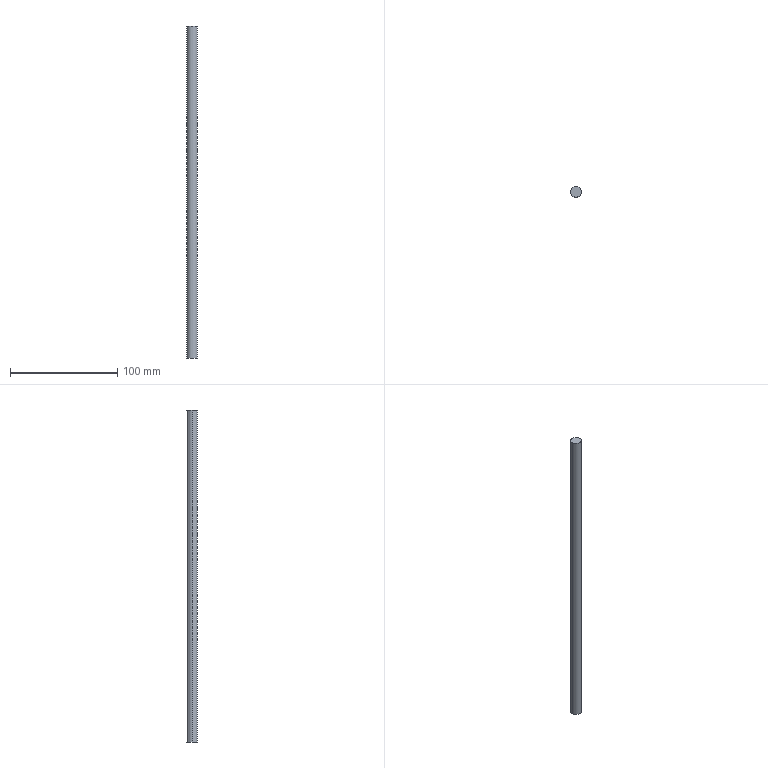Part | STEP file | 1 solid | 4 faces | box 10 x 10 x 310 mm | volume 24347 mm3 | cylinder 2 | plane 2 | commonest cylinder face diameters 10 x2
STEP:
#1=CARTESIAN_POINT('',(0.,0.,0.));
#2=DIRECTION('',(0.,0.,1.));
#3=DIRECTION('',(1.,0.,0.));
#4=AXIS2_PLACEMENT_3D('',#1,#2,#3);
#5=CARTESIAN_POINT('',(5.,0.,310.));
#6=VERTEX_POINT('',#5);
#7=CARTESIAN_POINT('',(-5.,0.,310.));
#8=VERTEX_POINT('',#7);
#9=CARTESIAN_POINT('',(0.,0.,310.));
#10=DIRECTION('',(0.,0.,1.));
#11=DIRECTION('',(1.,0.,0.));
#12=AXIS2_PLACEMENT_3D('',#9,#10,#11);
#13=CIRCLE('',#12,5.);
#14=CARTESIAN_POINT('',(0.,0.,310.));
#15=DIRECTION('',(0.,0.,-1.));
#16=DIRECTION('',(-1.,0.,0.));
#17=AXIS2_PLACEMENT_3D('',#14,#15,#16);
#18=CYLINDRICAL_SURFACE('',#17,5.);
#19=CARTESIAN_POINT('',(3.142,0.));
#20=DIRECTION('',(-1.,0.));
#21=VECTOR('',#20,1.);
#22=LINE('',#19,#21);
#23=(GEOMETRIC_REPRESENTATION_CONTEXT(2)PARAMETRIC_REPRESENTATION_CONTEXT()REPRESENTATION_CONTEXT('',''));
#24=DEFINITIONAL_REPRESENTATION('',(#22),#23);
#25=PCURVE('',#18,#24);
#26=CARTESIAN_POINT('',(0.,0.,310.));
#27=DIRECTION('',(0.,0.,1.));
#28=DIRECTION('',(1.,0.,0.));
#29=AXIS2_PLACEMENT_3D('',#26,#27,#28);
#30=PLANE('',#29);
#31=CARTESIAN_POINT('',(0.,0.));
#32=DIRECTION('',(1.,0.));
#33=AXIS2_PLACEMENT_2D('',#31,#32);
#34=CIRCLE('',#33,5.);
#35=(GEOMETRIC_REPRESENTATION_CONTEXT(2)PARAMETRIC_REPRESENTATION_CONTEXT()REPRESENTATION_CONTEXT('',''));
#36=DEFINITIONAL_REPRESENTATION('',(#34),#35);
#37=PCURVE('',#30,#36);
#38=SURFACE_CURVE('',#13,(#25,#37),.PCURVE_S1.);
#39=EDGE_CURVE('',#6,#8,#38,.T.);
#40=ORIENTED_EDGE('',*,*,#39,.F.);
#41=CARTESIAN_POINT('',(5.,0.,0.));
#42=VERTEX_POINT('',#41);
#43=CARTESIAN_POINT('',(5.,0.,310.));
#44=DIRECTION('',(0.,0.,-1.));
#45=VECTOR('',#44,1.);
#46=LINE('',#43,#45);
#47=CARTESIAN_POINT('',(3.142,0.));
#48=DIRECTION('',(0.,1.));
#49=VECTOR('',#48,1.);
#50=LINE('',#47,#49);
#51=(GEOMETRIC_REPRESENTATION_CONTEXT(2)PARAMETRIC_REPRESENTATION_CONTEXT()REPRESENTATION_CONTEXT('',''));
#52=DEFINITIONAL_REPRESENTATION('',(#50),#51);
#53=PCURVE('',#18,#52);
#54=CARTESIAN_POINT('',(0.,0.,310.));
#55=DIRECTION('',(0.,0.,-1.));
#56=DIRECTION('',(-1.,0.,0.));
#57=AXIS2_PLACEMENT_3D('',#54,#55,#56);
#58=CYLINDRICAL_SURFACE('',#57,5.);
#59=CARTESIAN_POINT('',(3.142,0.));
#60=DIRECTION('',(0.,1.));
#61=VECTOR('',#60,1.);
#62=LINE('',#59,#61);
#63=(GEOMETRIC_REPRESENTATION_CONTEXT(2)PARAMETRIC_REPRESENTATION_CONTEXT()REPRESENTATION_CONTEXT('',''));
#64=DEFINITIONAL_REPRESENTATION('',(#62),#63);
#65=PCURVE('',#58,#64);
#66=SURFACE_CURVE('',#46,(#53,#65),.PCURVE_S1.);
#67=EDGE_CURVE('',#6,#42,#66,.T.);
#68=ORIENTED_EDGE('',*,*,#67,.T.);
#69=CARTESIAN_POINT('',(-5.,0.,0.));
#70=VERTEX_POINT('',#69);
#71=CARTESIAN_POINT('',(0.,0.,0.));
#72=DIRECTION('',(0.,0.,1.));
#73=DIRECTION('',(1.,0.,0.));
#74=AXIS2_PLACEMENT_3D('',#71,#72,#73);
#75=CIRCLE('',#74,5.);
#76=CARTESIAN_POINT('',(3.142,310.));
#77=DIRECTION('',(-1.,0.));
#78=VECTOR('',#77,1.);
#79=LINE('',#76,#78);
#80=(GEOMETRIC_REPRESENTATION_CONTEXT(2)PARAMETRIC_REPRESENTATION_CONTEXT()REPRESENTATION_CONTEXT('',''));
#81=DEFINITIONAL_REPRESENTATION('',(#79),#80);
#82=PCURVE('',#18,#81);
#83=CARTESIAN_POINT('',(0.,0.,0.));
#84=DIRECTION('',(0.,0.,1.));
#85=DIRECTION('',(1.,0.,0.));
#86=AXIS2_PLACEMENT_3D('',#83,#84,#85);
#87=PLANE('',#86);
#88=CARTESIAN_POINT('',(0.,0.));
#89=DIRECTION('',(1.,0.));
#90=AXIS2_PLACEMENT_2D('',#88,#89);
#91=CIRCLE('',#90,5.);
#92=(GEOMETRIC_REPRESENTATION_CONTEXT(2)PARAMETRIC_REPRESENTATION_CONTEXT()REPRESENTATION_CONTEXT('',''));
#93=DEFINITIONAL_REPRESENTATION('',(#91),#92);
#94=PCURVE('',#87,#93);
#95=SURFACE_CURVE('',#75,(#82,#94),.PCURVE_S1.);
#96=EDGE_CURVE('',#42,#70,#95,.T.);
#97=ORIENTED_EDGE('',*,*,#96,.T.);
#98=CARTESIAN_POINT('',(-5.,0.,310.));
#99=DIRECTION('',(0.,0.,-1.));
#100=VECTOR('',#99,1.);
#101=LINE('',#98,#100);
#102=CARTESIAN_POINT('',(0.,0.));
#103=DIRECTION('',(0.,1.));
#104=VECTOR('',#103,1.);
#105=LINE('',#102,#104);
#106=(GEOMETRIC_REPRESENTATION_CONTEXT(2)PARAMETRIC_REPRESENTATION_CONTEXT()REPRESENTATION_CONTEXT('',''));
#107=DEFINITIONAL_REPRESENTATION('',(#105),#106);
#108=PCURVE('',#18,#107);
#109=CARTESIAN_POINT('',(6.283,0.));
#110=DIRECTION('',(0.,1.));
#111=VECTOR('',#110,1.);
#112=LINE('',#109,#111);
#113=(GEOMETRIC_REPRESENTATION_CONTEXT(2)PARAMETRIC_REPRESENTATION_CONTEXT()REPRESENTATION_CONTEXT('',''));
#114=DEFINITIONAL_REPRESENTATION('',(#112),#113);
#115=PCURVE('',#58,#114);
#116=SURFACE_CURVE('',#101,(#108,#115),.PCURVE_S1.);
#117=EDGE_CURVE('',#8,#70,#116,.T.);
#118=ORIENTED_EDGE('',*,*,#117,.F.);
#119=EDGE_LOOP('',(#40,#68,#97,#118));
#120=FACE_BOUND('',#119,.T.);
#121=ADVANCED_FACE('',(#120),#18,.T.);
#122=ORIENTED_EDGE('',*,*,#67,.F.);
#123=CARTESIAN_POINT('',(0.,0.,310.));
#124=DIRECTION('',(0.,0.,1.));
#125=DIRECTION('',(1.,0.,0.));
#126=AXIS2_PLACEMENT_3D('',#123,#124,#125);
#127=CIRCLE('',#126,5.);
#128=CARTESIAN_POINT('',(9.425,0.));
#129=DIRECTION('',(-1.,0.));
#130=VECTOR('',#129,1.);
#131=LINE('',#128,#130);
#132=(GEOMETRIC_REPRESENTATION_CONTEXT(2)PARAMETRIC_REPRESENTATION_CONTEXT()REPRESENTATION_CONTEXT('',''));
#133=DEFINITIONAL_REPRESENTATION('',(#131),#132);
#134=PCURVE('',#58,#133);
#135=CARTESIAN_POINT('',(0.,0.));
#136=DIRECTION('',(1.,0.));
#137=AXIS2_PLACEMENT_2D('',#135,#136);
#138=CIRCLE('',#137,5.);
#139=(GEOMETRIC_REPRESENTATION_CONTEXT(2)PARAMETRIC_REPRESENTATION_CONTEXT()REPRESENTATION_CONTEXT('',''));
#140=DEFINITIONAL_REPRESENTATION('',(#138),#139);
#141=PCURVE('',#30,#140);
#142=SURFACE_CURVE('',#127,(#134,#141),.PCURVE_S1.);
#143=EDGE_CURVE('',#8,#6,#142,.T.);
#144=ORIENTED_EDGE('',*,*,#143,.F.);
#145=ORIENTED_EDGE('',*,*,#117,.T.);
#146=CARTESIAN_POINT('',(0.,0.,0.));
#147=DIRECTION('',(0.,0.,1.));
#148=DIRECTION('',(1.,0.,0.));
#149=AXIS2_PLACEMENT_3D('',#146,#147,#148);
#150=CIRCLE('',#149,5.);
#151=CARTESIAN_POINT('',(9.425,310.));
#152=DIRECTION('',(-1.,0.));
#153=VECTOR('',#152,1.);
#154=LINE('',#151,#153);
#155=(GEOMETRIC_REPRESENTATION_CONTEXT(2)PARAMETRIC_REPRESENTATION_CONTEXT()REPRESENTATION_CONTEXT('',''));
#156=DEFINITIONAL_REPRESENTATION('',(#154),#155);
#157=PCURVE('',#58,#156);
#158=CARTESIAN_POINT('',(0.,0.));
#159=DIRECTION('',(1.,0.));
#160=AXIS2_PLACEMENT_2D('',#158,#159);
#161=CIRCLE('',#160,5.);
#162=(GEOMETRIC_REPRESENTATION_CONTEXT(2)PARAMETRIC_REPRESENTATION_CONTEXT()REPRESENTATION_CONTEXT('',''));
#163=DEFINITIONAL_REPRESENTATION('',(#161),#162);
#164=PCURVE('',#87,#163);
#165=SURFACE_CURVE('',#150,(#157,#164),.PCURVE_S1.);
#166=EDGE_CURVE('',#70,#42,#165,.T.);
#167=ORIENTED_EDGE('',*,*,#166,.T.);
#168=EDGE_LOOP('',(#122,#144,#145,#167));
#169=FACE_BOUND('',#168,.T.);
#170=ADVANCED_FACE('',(#169),#58,.T.);
#171=ORIENTED_EDGE('',*,*,#143,.T.);
#172=ORIENTED_EDGE('',*,*,#39,.T.);
#173=EDGE_LOOP('',(#171,#172));
#174=FACE_BOUND('',#173,.T.);
#175=ADVANCED_FACE('',(#174),#30,.T.);
#176=ORIENTED_EDGE('',*,*,#166,.F.);
#177=ORIENTED_EDGE('',*,*,#96,.F.);
#178=EDGE_LOOP('',(#176,#177));
#179=FACE_BOUND('',#178,.T.);
#180=ADVANCED_FACE('',(#179),#87,.F.);
#181=CLOSED_SHELL('',(#121,#170,#175,#180));
#182=MANIFOLD_SOLID_BREP('',#181);
#183=(LENGTH_UNIT()NAMED_UNIT(*)SI_UNIT(.MILLI.,.METRE.));
#184=UNCERTAINTY_MEASURE_WITH_UNIT(LENGTH_MEASURE(0.0000001),#183,'','');
#185=(NAMED_UNIT(*)PLANE_ANGLE_UNIT()SI_UNIT($,.RADIAN.));
#186=(NAMED_UNIT(*)SI_UNIT($,.STERADIAN.)SOLID_ANGLE_UNIT());
#187=(GEOMETRIC_REPRESENTATION_CONTEXT(3)GLOBAL_UNCERTAINTY_ASSIGNED_CONTEXT((#184))GLOBAL_UNIT_ASSIGNED_CONTEXT((#183,#185,#186))REPRESENTATION_CONTEXT('',''));
#188=ADVANCED_BREP_SHAPE_REPRESENTATION('',(#4,#182),#187);